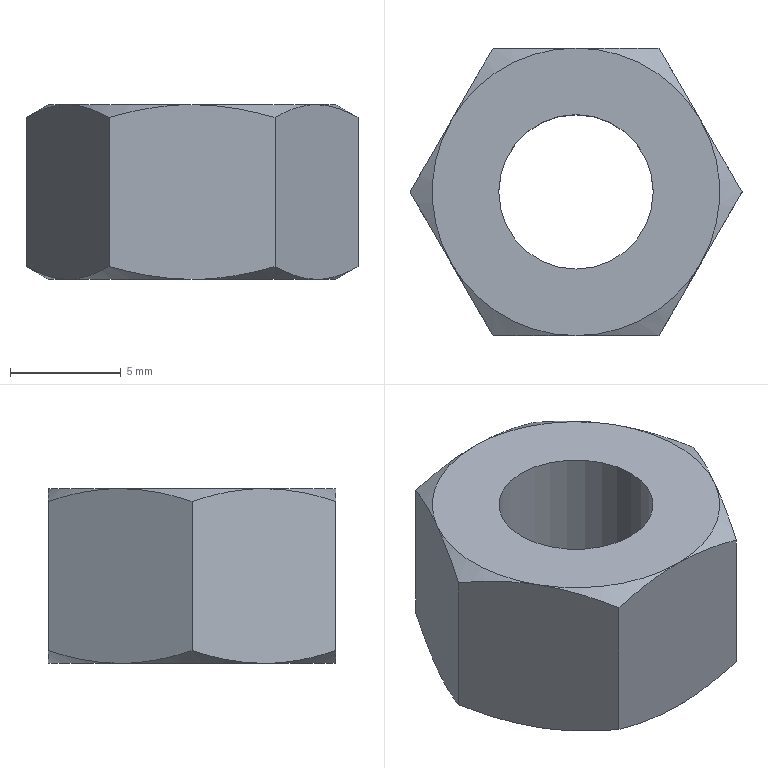Part | STEP file | 冲床-300配套压波_id202_x_t | 1 solid | 21 faces | box 15.011 x 13 x 7.9 mm | volume 848.643 mm3 | cone 12 | plane 8 | cylinder 1 | commonest cylinder face diameters 6.985 x1
STEP:
#1=CARTESIAN_POINT('',(1810.629,-81.75,123.));
#2=VERTEX_POINT('',#1);
#3=CARTESIAN_POINT('',(1805.,-78.5,123.));
#4=VERTEX_POINT('',#3);
#5=CARTESIAN_POINT('',(1805.,-85.,123.));
#6=DIRECTION('',(0.,0.,1.));
#7=DIRECTION('',(1.,0.,0.));
#8=AXIS2_PLACEMENT_3D('',#5,#6,#7);
#9=CIRCLE('',#8,6.5);
#10=EDGE_CURVE('',#2,#4,#9,.T.);
#11=ORIENTED_EDGE('',*,*,#10,.F.);
#12=CARTESIAN_POINT('',(1810.629,-88.25,123.));
#13=VERTEX_POINT('',#12);
#14=CARTESIAN_POINT('',(1805.,-85.,123.));
#15=DIRECTION('',(0.,0.,1.));
#16=DIRECTION('',(1.,0.,0.));
#17=AXIS2_PLACEMENT_3D('',#14,#15,#16);
#18=CIRCLE('',#17,6.5);
#19=EDGE_CURVE('',#13,#2,#18,.T.);
#20=ORIENTED_EDGE('',*,*,#19,.F.);
#21=CARTESIAN_POINT('',(1805.,-91.5,123.));
#22=VERTEX_POINT('',#21);
#23=CARTESIAN_POINT('',(1805.,-85.,123.));
#24=DIRECTION('',(0.,0.,1.));
#25=DIRECTION('',(1.,0.,0.));
#26=AXIS2_PLACEMENT_3D('',#23,#24,#25);
#27=CIRCLE('',#26,6.5);
#28=EDGE_CURVE('',#22,#13,#27,.T.);
#29=ORIENTED_EDGE('',*,*,#28,.F.);
#30=CARTESIAN_POINT('',(1799.371,-88.25,123.));
#31=VERTEX_POINT('',#30);
#32=CARTESIAN_POINT('',(1805.,-85.,123.));
#33=DIRECTION('',(0.,0.,1.));
#34=DIRECTION('',(1.,0.,0.));
#35=AXIS2_PLACEMENT_3D('',#32,#33,#34);
#36=CIRCLE('',#35,6.5);
#37=EDGE_CURVE('',#31,#22,#36,.T.);
#38=ORIENTED_EDGE('',*,*,#37,.F.);
#39=CARTESIAN_POINT('',(1799.371,-81.75,123.));
#40=VERTEX_POINT('',#39);
#41=CARTESIAN_POINT('',(1805.,-85.,123.));
#42=DIRECTION('',(0.,0.,1.));
#43=DIRECTION('',(1.,0.,0.));
#44=AXIS2_PLACEMENT_3D('',#41,#42,#43);
#45=CIRCLE('',#44,6.5);
#46=EDGE_CURVE('',#40,#31,#45,.T.);
#47=ORIENTED_EDGE('',*,*,#46,.F.);
#48=CARTESIAN_POINT('',(1805.,-85.,123.));
#49=DIRECTION('',(0.,0.,1.));
#50=DIRECTION('',(1.,0.,0.));
#51=AXIS2_PLACEMENT_3D('',#48,#49,#50);
#52=CIRCLE('',#51,6.5);
#53=EDGE_CURVE('',#4,#40,#52,.T.);
#54=ORIENTED_EDGE('',*,*,#53,.F.);
#55=EDGE_LOOP('',(#11,#20,#29,#38,#47,#54));
#56=FACE_BOUND('',#55,.T.);
#57=CARTESIAN_POINT('',(1801.507,-85.,123.));
#58=VERTEX_POINT('',#57);
#59=CARTESIAN_POINT('',(1805.,-85.,123.));
#60=DIRECTION('',(0.,0.,1.));
#61=DIRECTION('',(-1.,0.,0.));
#62=AXIS2_PLACEMENT_3D('',#59,#60,#61);
#63=CIRCLE('',#62,3.493);
#64=EDGE_CURVE('',#58,#58,#63,.T.);
#65=ORIENTED_EDGE('',*,*,#64,.T.);
#66=EDGE_LOOP('',(#65));
#67=FACE_BOUND('',#66,.T.);
#68=CARTESIAN_POINT('',(1805.,-72.,123.));
#69=DIRECTION('',(0.,0.,-1.));
#70=DIRECTION('',(-1.,0.,0.));
#71=AXIS2_PLACEMENT_3D('',#68,#69,#70);
#72=PLANE('',#71);
#73=ADVANCED_FACE('',(#56,#67),#72,.T.);
#74=CARTESIAN_POINT('',(1810.629,-88.25,130.9));
#75=VERTEX_POINT('',#74);
#76=CARTESIAN_POINT('',(1810.629,-81.75,130.9));
#77=VERTEX_POINT('',#76);
#78=CARTESIAN_POINT('',(1805.,-85.,130.9));
#79=DIRECTION('',(0.,0.,1.));
#80=DIRECTION('',(1.,0.,0.));
#81=AXIS2_PLACEMENT_3D('',#78,#79,#80);
#82=CIRCLE('',#81,6.5);
#83=EDGE_CURVE('',#75,#77,#82,.T.);
#84=ORIENTED_EDGE('',*,*,#83,.T.);
#85=CARTESIAN_POINT('',(1805.,-78.5,130.9));
#86=VERTEX_POINT('',#85);
#87=CARTESIAN_POINT('',(1805.,-85.,130.9));
#88=DIRECTION('',(0.,0.,1.));
#89=DIRECTION('',(1.,0.,0.));
#90=AXIS2_PLACEMENT_3D('',#87,#88,#89);
#91=CIRCLE('',#90,6.5);
#92=EDGE_CURVE('',#77,#86,#91,.T.);
#93=ORIENTED_EDGE('',*,*,#92,.T.);
#94=CARTESIAN_POINT('',(1799.371,-81.75,130.9));
#95=VERTEX_POINT('',#94);
#96=CARTESIAN_POINT('',(1805.,-85.,130.9));
#97=DIRECTION('',(0.,0.,1.));
#98=DIRECTION('',(1.,0.,0.));
#99=AXIS2_PLACEMENT_3D('',#96,#97,#98);
#100=CIRCLE('',#99,6.5);
#101=EDGE_CURVE('',#86,#95,#100,.T.);
#102=ORIENTED_EDGE('',*,*,#101,.T.);
#103=CARTESIAN_POINT('',(1799.371,-88.25,130.9));
#104=VERTEX_POINT('',#103);
#105=CARTESIAN_POINT('',(1805.,-85.,130.9));
#106=DIRECTION('',(0.,0.,1.));
#107=DIRECTION('',(1.,0.,0.));
#108=AXIS2_PLACEMENT_3D('',#105,#106,#107);
#109=CIRCLE('',#108,6.5);
#110=EDGE_CURVE('',#95,#104,#109,.T.);
#111=ORIENTED_EDGE('',*,*,#110,.T.);
#112=CARTESIAN_POINT('',(1805.,-91.5,130.9));
#113=VERTEX_POINT('',#112);
#114=CARTESIAN_POINT('',(1805.,-85.,130.9));
#115=DIRECTION('',(0.,0.,1.));
#116=DIRECTION('',(1.,0.,0.));
#117=AXIS2_PLACEMENT_3D('',#114,#115,#116);
#118=CIRCLE('',#117,6.5);
#119=EDGE_CURVE('',#104,#113,#118,.T.);
#120=ORIENTED_EDGE('',*,*,#119,.T.);
#121=CARTESIAN_POINT('',(1805.,-85.,130.9));
#122=DIRECTION('',(0.,0.,1.));
#123=DIRECTION('',(1.,0.,0.));
#124=AXIS2_PLACEMENT_3D('',#121,#122,#123);
#125=CIRCLE('',#124,6.5);
#126=EDGE_CURVE('',#113,#75,#125,.T.);
#127=ORIENTED_EDGE('',*,*,#126,.T.);
#128=EDGE_LOOP('',(#84,#93,#102,#111,#120,#127));
#129=FACE_BOUND('',#128,.T.);
#130=CARTESIAN_POINT('',(1801.507,-85.,130.9));
#131=VERTEX_POINT('',#130);
#132=CARTESIAN_POINT('',(1805.,-85.,130.9));
#133=DIRECTION('',(0.,0.,1.));
#134=DIRECTION('',(-1.,0.,0.));
#135=AXIS2_PLACEMENT_3D('',#132,#133,#134);
#136=CIRCLE('',#135,3.493);
#137=EDGE_CURVE('',#131,#131,#136,.T.);
#138=ORIENTED_EDGE('',*,*,#137,.F.);
#139=EDGE_LOOP('',(#138));
#140=FACE_BOUND('',#139,.T.);
#141=CARTESIAN_POINT('',(1805.,-72.,130.9));
#142=DIRECTION('',(0.,0.,-1.));
#143=DIRECTION('',(-1.,0.,0.));
#144=AXIS2_PLACEMENT_3D('',#141,#142,#143);
#145=PLANE('',#144);
#146=ADVANCED_FACE('',(#129,#140),#145,.F.);
#147=CARTESIAN_POINT('',(1797.494,-85.,123.581));
#148=VERTEX_POINT('',#147);
#149=CARTESIAN_POINT('',(1797.494,-85.,130.319));
#150=VERTEX_POINT('',#149);
#151=CARTESIAN_POINT('',(1797.494,-85.,123.));
#152=DIRECTION('',(0.,0.,1.));
#153=VECTOR('',#152,1.);
#154=LINE('',#151,#153);
#155=EDGE_CURVE('',#148,#150,#154,.T.);
#156=ORIENTED_EDGE('',*,*,#155,.T.);
#157=CARTESIAN_POINT('',(1797.494,-85.,130.319));
#158=CARTESIAN_POINT('',(1798.108,-83.937,130.674));
#159=CARTESIAN_POINT('',(1798.731,-82.857,130.9));
#160=CARTESIAN_POINT('',(1799.371,-81.75,130.9));
#161=B_SPLINE_CURVE_WITH_KNOTS('',3,(#157,#158,#159,#160),.UNSPECIFIED.,.F.,.F.,(4,4),(0.,1.),.UNSPECIFIED.);
#162=EDGE_CURVE('',#150,#95,#161,.T.);
#163=ORIENTED_EDGE('',*,*,#162,.T.);
#164=CARTESIAN_POINT('',(1801.247,-78.5,130.319));
#165=VERTEX_POINT('',#164);
#166=CARTESIAN_POINT('',(1799.371,-81.75,130.9));
#167=CARTESIAN_POINT('',(1800.008,-80.647,130.9));
#168=CARTESIAN_POINT('',(1800.635,-79.561,130.673));
#169=CARTESIAN_POINT('',(1801.247,-78.5,130.319));
#170=B_SPLINE_CURVE_WITH_KNOTS('',3,(#166,#167,#168,#169),.UNSPECIFIED.,.F.,.F.,(4,4),(0.,1.),.UNSPECIFIED.);
#171=EDGE_CURVE('',#95,#165,#170,.T.);
#172=ORIENTED_EDGE('',*,*,#171,.T.);
#173=CARTESIAN_POINT('',(1801.247,-78.5,123.581));
#174=VERTEX_POINT('',#173);
#175=CARTESIAN_POINT('',(1801.247,-78.5,123.));
#176=DIRECTION('',(0.,0.,1.));
#177=VECTOR('',#176,1.);
#178=LINE('',#175,#177);
#179=EDGE_CURVE('',#174,#165,#178,.T.);
#180=ORIENTED_EDGE('',*,*,#179,.F.);
#181=CARTESIAN_POINT('',(1801.247,-78.5,123.581));
#182=CARTESIAN_POINT('',(1800.633,-79.563,123.226));
#183=CARTESIAN_POINT('',(1800.01,-80.643,123.));
#184=CARTESIAN_POINT('',(1799.371,-81.75,123.));
#185=B_SPLINE_CURVE_WITH_KNOTS('',3,(#181,#182,#183,#184),.UNSPECIFIED.,.F.,.F.,(4,4),(0.,1.),.UNSPECIFIED.);
#186=EDGE_CURVE('',#174,#40,#185,.T.);
#187=ORIENTED_EDGE('',*,*,#186,.T.);
#188=CARTESIAN_POINT('',(1799.371,-81.75,123.));
#189=CARTESIAN_POINT('',(1798.734,-82.853,123.));
#190=CARTESIAN_POINT('',(1798.107,-83.939,123.227));
#191=CARTESIAN_POINT('',(1797.494,-85.,123.581));
#192=B_SPLINE_CURVE_WITH_KNOTS('',3,(#188,#189,#190,#191),.UNSPECIFIED.,.F.,.F.,(4,4),(0.,1.),.UNSPECIFIED.);
#193=EDGE_CURVE('',#40,#148,#192,.T.);
#194=ORIENTED_EDGE('',*,*,#193,.T.);
#195=EDGE_LOOP('',(#156,#163,#172,#180,#187,#194));
#196=FACE_OUTER_BOUND('',#195,.T.);
#197=CARTESIAN_POINT('',(1801.247,-78.5,123.));
#198=DIRECTION('',(-0.866,0.5,0.));
#199=DIRECTION('',(0.5,0.866,0.));
#200=AXIS2_PLACEMENT_3D('',#197,#198,#199);
#201=PLANE('',#200);
#202=ADVANCED_FACE('',(#196),#201,.T.);
#203=CARTESIAN_POINT('',(1801.247,-91.5,123.581));
#204=VERTEX_POINT('',#203);
#205=CARTESIAN_POINT('',(1801.247,-91.5,130.319));
#206=VERTEX_POINT('',#205);
#207=CARTESIAN_POINT('',(1801.247,-91.5,123.));
#208=DIRECTION('',(0.,0.,1.));
#209=VECTOR('',#208,1.);
#210=LINE('',#207,#209);
#211=EDGE_CURVE('',#204,#206,#210,.T.);
#212=ORIENTED_EDGE('',*,*,#211,.T.);
#213=CARTESIAN_POINT('',(1801.247,-91.5,130.319));
#214=CARTESIAN_POINT('',(1800.633,-90.437,130.674));
#215=CARTESIAN_POINT('',(1800.01,-89.357,130.9));
#216=CARTESIAN_POINT('',(1799.371,-88.25,130.9));
#217=B_SPLINE_CURVE_WITH_KNOTS('',3,(#213,#214,#215,#216),.UNSPECIFIED.,.F.,.F.,(4,4),(0.,1.),.UNSPECIFIED.);
#218=EDGE_CURVE('',#206,#104,#217,.T.);
#219=ORIENTED_EDGE('',*,*,#218,.T.);
#220=CARTESIAN_POINT('',(1799.371,-88.25,130.9));
#221=CARTESIAN_POINT('',(1798.734,-87.147,130.9));
#222=CARTESIAN_POINT('',(1798.107,-86.061,130.673));
#223=CARTESIAN_POINT('',(1797.494,-85.,130.319));
#224=B_SPLINE_CURVE_WITH_KNOTS('',3,(#220,#221,#222,#223),.UNSPECIFIED.,.F.,.F.,(4,4),(0.,1.),.UNSPECIFIED.);
#225=EDGE_CURVE('',#104,#150,#224,.T.);
#226=ORIENTED_EDGE('',*,*,#225,.T.);
#227=ORIENTED_EDGE('',*,*,#155,.F.);
#228=CARTESIAN_POINT('',(1797.494,-85.,123.581));
#229=CARTESIAN_POINT('',(1798.108,-86.063,123.226));
#230=CARTESIAN_POINT('',(1798.731,-87.143,123.));
#231=CARTESIAN_POINT('',(1799.371,-88.25,123.));
#232=B_SPLINE_CURVE_WITH_KNOTS('',3,(#228,#229,#230,#231),.UNSPECIFIED.,.F.,.F.,(4,4),(0.,1.),.UNSPECIFIED.);
#233=EDGE_CURVE('',#148,#31,#232,.T.);
#234=ORIENTED_EDGE('',*,*,#233,.T.);
#235=CARTESIAN_POINT('',(1799.371,-88.25,123.));
#236=CARTESIAN_POINT('',(1800.008,-89.353,123.));
#237=CARTESIAN_POINT('',(1800.635,-90.439,123.227));
#238=CARTESIAN_POINT('',(1801.247,-91.5,123.581));
#239=B_SPLINE_CURVE_WITH_KNOTS('',3,(#235,#236,#237,#238),.UNSPECIFIED.,.F.,.F.,(4,4),(0.,1.),.UNSPECIFIED.);
#240=EDGE_CURVE('',#31,#204,#239,.T.);
#241=ORIENTED_EDGE('',*,*,#240,.T.);
#242=EDGE_LOOP('',(#212,#219,#226,#227,#234,#241));
#243=FACE_OUTER_BOUND('',#242,.T.);
#244=CARTESIAN_POINT('',(1797.494,-85.,123.));
#245=DIRECTION('',(-0.866,-0.5,0.));
#246=DIRECTION('',(-0.5,0.866,0.));
#247=AXIS2_PLACEMENT_3D('',#244,#245,#246);
#248=PLANE('',#247);
#249=ADVANCED_FACE('',(#243),#248,.T.);
#250=CARTESIAN_POINT('',(1808.753,-91.5,123.581));
#251=VERTEX_POINT('',#250);
#252=CARTESIAN_POINT('',(1808.753,-91.5,130.319));
#253=VERTEX_POINT('',#252);
#254=CARTESIAN_POINT('',(1808.753,-91.5,123.));
#255=DIRECTION('',(0.,0.,1.));
#256=VECTOR('',#255,1.);
#257=LINE('',#254,#256);
#258=EDGE_CURVE('',#251,#253,#257,.T.);
#259=ORIENTED_EDGE('',*,*,#258,.T.);
#260=CARTESIAN_POINT('',(1808.753,-91.5,130.319));
#261=CARTESIAN_POINT('',(1807.532,-91.5,130.672));
#262=CARTESIAN_POINT('',(1806.268,-91.5,130.9));
#263=CARTESIAN_POINT('',(1805.,-91.5,130.9));
#264=B_SPLINE_CURVE_WITH_KNOTS('',3,(#260,#261,#262,#263),.UNSPECIFIED.,.F.,.F.,(4,4),(0.,1.),.UNSPECIFIED.);
#265=EDGE_CURVE('',#253,#113,#264,.T.);
#266=ORIENTED_EDGE('',*,*,#265,.T.);
#267=CARTESIAN_POINT('',(1805.,-91.5,130.9));
#268=CARTESIAN_POINT('',(1803.731,-91.5,130.9));
#269=CARTESIAN_POINT('',(1802.461,-91.5,130.67));
#270=CARTESIAN_POINT('',(1801.247,-91.5,130.319));
#271=B_SPLINE_CURVE_WITH_KNOTS('',3,(#267,#268,#269,#270),.UNSPECIFIED.,.F.,.F.,(4,4),(0.,1.),.UNSPECIFIED.);
#272=EDGE_CURVE('',#113,#206,#271,.T.);
#273=ORIENTED_EDGE('',*,*,#272,.T.);
#274=ORIENTED_EDGE('',*,*,#211,.F.);
#275=CARTESIAN_POINT('',(1801.247,-91.5,123.581));
#276=CARTESIAN_POINT('',(1802.461,-91.5,123.23));
#277=CARTESIAN_POINT('',(1803.731,-91.5,123.));
#278=CARTESIAN_POINT('',(1805.,-91.5,123.));
#279=B_SPLINE_CURVE_WITH_KNOTS('',3,(#275,#276,#277,#278),.UNSPECIFIED.,.F.,.F.,(4,4),(0.,1.),.UNSPECIFIED.);
#280=EDGE_CURVE('',#204,#22,#279,.T.);
#281=ORIENTED_EDGE('',*,*,#280,.T.);
#282=CARTESIAN_POINT('',(1805.,-91.5,123.));
#283=CARTESIAN_POINT('',(1806.268,-91.5,123.));
#284=CARTESIAN_POINT('',(1807.532,-91.5,123.228));
#285=CARTESIAN_POINT('',(1808.753,-91.5,123.581));
#286=B_SPLINE_CURVE_WITH_KNOTS('',3,(#282,#283,#284,#285),.UNSPECIFIED.,.F.,.F.,(4,4),(0.,1.),.UNSPECIFIED.);
#287=EDGE_CURVE('',#22,#251,#286,.T.);
#288=ORIENTED_EDGE('',*,*,#287,.T.);
#289=EDGE_LOOP('',(#259,#266,#273,#274,#281,#288));
#290=FACE_OUTER_BOUND('',#289,.T.);
#291=CARTESIAN_POINT('',(1801.247,-91.5,123.));
#292=DIRECTION('',(0.,-1.,0.));
#293=DIRECTION('',(0.,0.,1.));
#294=AXIS2_PLACEMENT_3D('',#291,#292,#293);
#295=PLANE('',#294);
#296=ADVANCED_FACE('',(#290),#295,.T.);
#297=CARTESIAN_POINT('',(1812.506,-85.,123.581));
#298=VERTEX_POINT('',#297);
#299=CARTESIAN_POINT('',(1812.506,-85.,130.319));
#300=VERTEX_POINT('',#299);
#301=CARTESIAN_POINT('',(1812.506,-85.,123.));
#302=DIRECTION('',(0.,0.,1.));
#303=VECTOR('',#302,1.);
#304=LINE('',#301,#303);
#305=EDGE_CURVE('',#298,#300,#304,.T.);
#306=ORIENTED_EDGE('',*,*,#305,.T.);
#307=CARTESIAN_POINT('',(1812.506,-85.,130.319));
#308=CARTESIAN_POINT('',(1811.892,-86.063,130.674));
#309=CARTESIAN_POINT('',(1811.269,-87.143,130.9));
#310=CARTESIAN_POINT('',(1810.629,-88.25,130.9));
#311=B_SPLINE_CURVE_WITH_KNOTS('',3,(#307,#308,#309,#310),.UNSPECIFIED.,.F.,.F.,(4,4),(0.,1.),.UNSPECIFIED.);
#312=EDGE_CURVE('',#300,#75,#311,.T.);
#313=ORIENTED_EDGE('',*,*,#312,.T.);
#314=CARTESIAN_POINT('',(1810.629,-88.25,130.9));
#315=CARTESIAN_POINT('',(1809.992,-89.353,130.9));
#316=CARTESIAN_POINT('',(1809.365,-90.439,130.673));
#317=CARTESIAN_POINT('',(1808.753,-91.5,130.319));
#318=B_SPLINE_CURVE_WITH_KNOTS('',3,(#314,#315,#316,#317),.UNSPECIFIED.,.F.,.F.,(4,4),(0.,1.),.UNSPECIFIED.);
#319=EDGE_CURVE('',#75,#253,#318,.T.);
#320=ORIENTED_EDGE('',*,*,#319,.T.);
#321=ORIENTED_EDGE('',*,*,#258,.F.);
#322=CARTESIAN_POINT('',(1808.753,-91.5,123.581));
#323=CARTESIAN_POINT('',(1809.367,-90.437,123.226));
#324=CARTESIAN_POINT('',(1809.99,-89.357,123.));
#325=CARTESIAN_POINT('',(1810.629,-88.25,123.));
#326=B_SPLINE_CURVE_WITH_KNOTS('',3,(#322,#323,#324,#325),.UNSPECIFIED.,.F.,.F.,(4,4),(0.,1.),.UNSPECIFIED.);
#327=EDGE_CURVE('',#251,#13,#326,.T.);
#328=ORIENTED_EDGE('',*,*,#327,.T.);
#329=CARTESIAN_POINT('',(1810.629,-88.25,123.));
#330=CARTESIAN_POINT('',(1811.266,-87.147,123.));
#331=CARTESIAN_POINT('',(1811.893,-86.061,123.227));
#332=CARTESIAN_POINT('',(1812.506,-85.,123.581));
#333=B_SPLINE_CURVE_WITH_KNOTS('',3,(#329,#330,#331,#332),.UNSPECIFIED.,.F.,.F.,(4,4),(0.,1.),.UNSPECIFIED.);
#334=EDGE_CURVE('',#13,#298,#333,.T.);
#335=ORIENTED_EDGE('',*,*,#334,.T.);
#336=EDGE_LOOP('',(#306,#313,#320,#321,#328,#335));
#337=FACE_OUTER_BOUND('',#336,.T.);
#338=CARTESIAN_POINT('',(1808.753,-91.5,123.));
#339=DIRECTION('',(0.866,-0.5,0.));
#340=DIRECTION('',(-0.5,-0.866,0.));
#341=AXIS2_PLACEMENT_3D('',#338,#339,#340);
#342=PLANE('',#341);
#343=ADVANCED_FACE('',(#337),#342,.T.);
#344=CARTESIAN_POINT('',(1808.753,-78.5,123.581));
#345=VERTEX_POINT('',#344);
#346=CARTESIAN_POINT('',(1808.753,-78.5,130.319));
#347=VERTEX_POINT('',#346);
#348=CARTESIAN_POINT('',(1808.753,-78.5,123.));
#349=DIRECTION('',(0.,0.,1.));
#350=VECTOR('',#349,1.);
#351=LINE('',#348,#350);
#352=EDGE_CURVE('',#345,#347,#351,.T.);
#353=ORIENTED_EDGE('',*,*,#352,.T.);
#354=CARTESIAN_POINT('',(1808.753,-78.5,130.319));
#355=CARTESIAN_POINT('',(1809.367,-79.563,130.674));
#356=CARTESIAN_POINT('',(1809.99,-80.643,130.9));
#357=CARTESIAN_POINT('',(1810.629,-81.75,130.9));
#358=B_SPLINE_CURVE_WITH_KNOTS('',3,(#354,#355,#356,#357),.UNSPECIFIED.,.F.,.F.,(4,4),(0.,1.),.UNSPECIFIED.);
#359=EDGE_CURVE('',#347,#77,#358,.T.);
#360=ORIENTED_EDGE('',*,*,#359,.T.);
#361=CARTESIAN_POINT('',(1810.629,-81.75,130.9));
#362=CARTESIAN_POINT('',(1811.266,-82.853,130.9));
#363=CARTESIAN_POINT('',(1811.893,-83.939,130.673));
#364=CARTESIAN_POINT('',(1812.506,-85.,130.319));
#365=B_SPLINE_CURVE_WITH_KNOTS('',3,(#361,#362,#363,#364),.UNSPECIFIED.,.F.,.F.,(4,4),(0.,1.),.UNSPECIFIED.);
#366=EDGE_CURVE('',#77,#300,#365,.T.);
#367=ORIENTED_EDGE('',*,*,#366,.T.);
#368=ORIENTED_EDGE('',*,*,#305,.F.);
#369=CARTESIAN_POINT('',(1812.506,-85.,123.581));
#370=CARTESIAN_POINT('',(1811.892,-83.937,123.226));
#371=CARTESIAN_POINT('',(1811.269,-82.857,123.));
#372=CARTESIAN_POINT('',(1810.629,-81.75,123.));
#373=B_SPLINE_CURVE_WITH_KNOTS('',3,(#369,#370,#371,#372),.UNSPECIFIED.,.F.,.F.,(4,4),(0.,1.),.UNSPECIFIED.);
#374=EDGE_CURVE('',#298,#2,#373,.T.);
#375=ORIENTED_EDGE('',*,*,#374,.T.);
#376=CARTESIAN_POINT('',(1810.629,-81.75,123.));
#377=CARTESIAN_POINT('',(1809.992,-80.647,123.));
#378=CARTESIAN_POINT('',(1809.365,-79.561,123.227));
#379=CARTESIAN_POINT('',(1808.753,-78.5,123.581));
#380=B_SPLINE_CURVE_WITH_KNOTS('',3,(#376,#377,#378,#379),.UNSPECIFIED.,.F.,.F.,(4,4),(0.,1.),.UNSPECIFIED.);
#381=EDGE_CURVE('',#2,#345,#380,.T.);
#382=ORIENTED_EDGE('',*,*,#381,.T.);
#383=EDGE_LOOP('',(#353,#360,#367,#368,#375,#382));
#384=FACE_OUTER_BOUND('',#383,.T.);
#385=CARTESIAN_POINT('',(1812.506,-85.,123.));
#386=DIRECTION('',(0.866,0.5,0.));
#387=DIRECTION('',(0.5,-0.866,0.));
#388=AXIS2_PLACEMENT_3D('',#385,#386,#387);
#389=PLANE('',#388);
#390=ADVANCED_FACE('',(#384),#389,.T.);
#391=ORIENTED_EDGE('',*,*,#179,.T.);
#392=CARTESIAN_POINT('',(1801.247,-78.5,130.319));
#393=CARTESIAN_POINT('',(1802.461,-78.5,130.67));
#394=CARTESIAN_POINT('',(1803.731,-78.5,130.9));
#395=CARTESIAN_POINT('',(1805.,-78.5,130.9));
#396=B_SPLINE_CURVE_WITH_KNOTS('',3,(#392,#393,#394,#395),.UNSPECIFIED.,.F.,.F.,(4,4),(0.,1.),.UNSPECIFIED.);
#397=EDGE_CURVE('',#165,#86,#396,.T.);
#398=ORIENTED_EDGE('',*,*,#397,.T.);
#399=CARTESIAN_POINT('',(1805.,-78.5,130.9));
#400=CARTESIAN_POINT('',(1806.268,-78.5,130.9));
#401=CARTESIAN_POINT('',(1807.532,-78.5,130.672));
#402=CARTESIAN_POINT('',(1808.753,-78.5,130.319));
#403=B_SPLINE_CURVE_WITH_KNOTS('',3,(#399,#400,#401,#402),.UNSPECIFIED.,.F.,.F.,(4,4),(0.,1.),.UNSPECIFIED.);
#404=EDGE_CURVE('',#86,#347,#403,.T.);
#405=ORIENTED_EDGE('',*,*,#404,.T.);
#406=ORIENTED_EDGE('',*,*,#352,.F.);
#407=CARTESIAN_POINT('',(1808.753,-78.5,123.581));
#408=CARTESIAN_POINT('',(1807.532,-78.5,123.228));
#409=CARTESIAN_POINT('',(1806.268,-78.5,123.));
#410=CARTESIAN_POINT('',(1805.,-78.5,123.));
#411=B_SPLINE_CURVE_WITH_KNOTS('',3,(#407,#408,#409,#410),.UNSPECIFIED.,.F.,.F.,(4,4),(0.,1.),.UNSPECIFIED.);
#412=EDGE_CURVE('',#345,#4,#411,.T.);
#413=ORIENTED_EDGE('',*,*,#412,.T.);
#414=CARTESIAN_POINT('',(1805.,-78.5,123.));
#415=CARTESIAN_POINT('',(1803.731,-78.5,123.));
#416=CARTESIAN_POINT('',(1802.461,-78.5,123.23));
#417=CARTESIAN_POINT('',(1801.247,-78.5,123.581));
#418=B_SPLINE_CURVE_WITH_KNOTS('',3,(#414,#415,#416,#417),.UNSPECIFIED.,.F.,.F.,(4,4),(0.,1.),.UNSPECIFIED.);
#419=EDGE_CURVE('',#4,#174,#418,.T.);
#420=ORIENTED_EDGE('',*,*,#419,.T.);
#421=EDGE_LOOP('',(#391,#398,#405,#406,#413,#420));
#422=FACE_OUTER_BOUND('',#421,.T.);
#423=CARTESIAN_POINT('',(1808.753,-78.5,123.));
#424=DIRECTION('',(0.,1.,0.));
#425=DIRECTION('',(0.,0.,-1.));
#426=AXIS2_PLACEMENT_3D('',#423,#424,#425);
#427=PLANE('',#426);
#428=ADVANCED_FACE('',(#422),#427,.T.);
#429=ORIENTED_EDGE('',*,*,#419,.F.);
#430=ORIENTED_EDGE('',*,*,#53,.T.);
#431=ORIENTED_EDGE('',*,*,#186,.F.);
#432=EDGE_LOOP('',(#429,#430,#431));
#433=FACE_OUTER_BOUND('',#432,.T.);
#434=CARTESIAN_POINT('',(1805.,-85.,123.581));
#435=DIRECTION('',(0.,0.,1.));
#436=DIRECTION('',(1.,0.,0.));
#437=AXIS2_PLACEMENT_3D('',#434,#435,#436);
#438=CONICAL_SURFACE('',#437,7.506,60.);
#439=ADVANCED_FACE('',(#433),#438,.T.);
#440=ORIENTED_EDGE('',*,*,#10,.T.);
#441=ORIENTED_EDGE('',*,*,#412,.F.);
#442=ORIENTED_EDGE('',*,*,#381,.F.);
#443=EDGE_LOOP('',(#440,#441,#442));
#444=FACE_OUTER_BOUND('',#443,.T.);
#445=CARTESIAN_POINT('',(1805.,-85.,123.581));
#446=DIRECTION('',(0.,0.,1.));
#447=DIRECTION('',(1.,0.,0.));
#448=AXIS2_PLACEMENT_3D('',#445,#446,#447);
#449=CONICAL_SURFACE('',#448,7.506,60.);
#450=ADVANCED_FACE('',(#444),#449,.T.);
#451=ORIENTED_EDGE('',*,*,#19,.T.);
#452=ORIENTED_EDGE('',*,*,#374,.F.);
#453=ORIENTED_EDGE('',*,*,#334,.F.);
#454=EDGE_LOOP('',(#451,#452,#453));
#455=FACE_OUTER_BOUND('',#454,.T.);
#456=CARTESIAN_POINT('',(1805.,-85.,123.581));
#457=DIRECTION('',(0.,0.,1.));
#458=DIRECTION('',(1.,0.,0.));
#459=AXIS2_PLACEMENT_3D('',#456,#457,#458);
#460=CONICAL_SURFACE('',#459,7.506,60.);
#461=ADVANCED_FACE('',(#455),#460,.T.);
#462=ORIENTED_EDGE('',*,*,#28,.T.);
#463=ORIENTED_EDGE('',*,*,#327,.F.);
#464=ORIENTED_EDGE('',*,*,#287,.F.);
#465=EDGE_LOOP('',(#462,#463,#464));
#466=FACE_OUTER_BOUND('',#465,.T.);
#467=CARTESIAN_POINT('',(1805.,-85.,123.581));
#468=DIRECTION('',(0.,0.,1.));
#469=DIRECTION('',(1.,0.,0.));
#470=AXIS2_PLACEMENT_3D('',#467,#468,#469);
#471=CONICAL_SURFACE('',#470,7.506,60.);
#472=ADVANCED_FACE('',(#466),#471,.T.);
#473=ORIENTED_EDGE('',*,*,#37,.T.);
#474=ORIENTED_EDGE('',*,*,#280,.F.);
#475=ORIENTED_EDGE('',*,*,#240,.F.);
#476=EDGE_LOOP('',(#473,#474,#475));
#477=FACE_OUTER_BOUND('',#476,.T.);
#478=CARTESIAN_POINT('',(1805.,-85.,123.581));
#479=DIRECTION('',(0.,0.,1.));
#480=DIRECTION('',(1.,0.,0.));
#481=AXIS2_PLACEMENT_3D('',#478,#479,#480);
#482=CONICAL_SURFACE('',#481,7.506,60.);
#483=ADVANCED_FACE('',(#477),#482,.T.);
#484=ORIENTED_EDGE('',*,*,#46,.T.);
#485=ORIENTED_EDGE('',*,*,#233,.F.);
#486=ORIENTED_EDGE('',*,*,#193,.F.);
#487=EDGE_LOOP('',(#484,#485,#486));
#488=FACE_OUTER_BOUND('',#487,.T.);
#489=CARTESIAN_POINT('',(1805.,-85.,123.581));
#490=DIRECTION('',(0.,0.,1.));
#491=DIRECTION('',(1.,0.,0.));
#492=AXIS2_PLACEMENT_3D('',#489,#490,#491);
#493=CONICAL_SURFACE('',#492,7.506,60.);
#494=ADVANCED_FACE('',(#488),#493,.T.);
#495=ORIENTED_EDGE('',*,*,#404,.F.);
#496=ORIENTED_EDGE('',*,*,#92,.F.);
#497=ORIENTED_EDGE('',*,*,#359,.F.);
#498=EDGE_LOOP('',(#495,#496,#497));
#499=FACE_OUTER_BOUND('',#498,.T.);
#500=CARTESIAN_POINT('',(1805.,-85.,130.9));
#501=DIRECTION('',(0.,0.,-1.));
#502=DIRECTION('',(-1.,0.,0.));
#503=AXIS2_PLACEMENT_3D('',#500,#501,#502);
#504=CONICAL_SURFACE('',#503,6.5,60.);
#505=ADVANCED_FACE('',(#499),#504,.T.);
#506=ORIENTED_EDGE('',*,*,#101,.F.);
#507=ORIENTED_EDGE('',*,*,#397,.F.);
#508=ORIENTED_EDGE('',*,*,#171,.F.);
#509=EDGE_LOOP('',(#506,#507,#508));
#510=FACE_OUTER_BOUND('',#509,.T.);
#511=CARTESIAN_POINT('',(1805.,-85.,130.9));
#512=DIRECTION('',(0.,0.,-1.));
#513=DIRECTION('',(-1.,0.,0.));
#514=AXIS2_PLACEMENT_3D('',#511,#512,#513);
#515=CONICAL_SURFACE('',#514,6.5,60.);
#516=ADVANCED_FACE('',(#510),#515,.T.);
#517=ORIENTED_EDGE('',*,*,#366,.F.);
#518=ORIENTED_EDGE('',*,*,#83,.F.);
#519=ORIENTED_EDGE('',*,*,#312,.F.);
#520=EDGE_LOOP('',(#517,#518,#519));
#521=FACE_OUTER_BOUND('',#520,.T.);
#522=CARTESIAN_POINT('',(1805.,-85.,130.9));
#523=DIRECTION('',(0.,0.,-1.));
#524=DIRECTION('',(-1.,0.,0.));
#525=AXIS2_PLACEMENT_3D('',#522,#523,#524);
#526=CONICAL_SURFACE('',#525,6.5,60.);
#527=ADVANCED_FACE('',(#521),#526,.T.);
#528=ORIENTED_EDGE('',*,*,#319,.F.);
#529=ORIENTED_EDGE('',*,*,#126,.F.);
#530=ORIENTED_EDGE('',*,*,#265,.F.);
#531=EDGE_LOOP('',(#528,#529,#530));
#532=FACE_OUTER_BOUND('',#531,.T.);
#533=CARTESIAN_POINT('',(1805.,-85.,130.9));
#534=DIRECTION('',(0.,0.,-1.));
#535=DIRECTION('',(-1.,0.,0.));
#536=AXIS2_PLACEMENT_3D('',#533,#534,#535);
#537=CONICAL_SURFACE('',#536,6.5,60.);
#538=ADVANCED_FACE('',(#532),#537,.T.);
#539=ORIENTED_EDGE('',*,*,#119,.F.);
#540=ORIENTED_EDGE('',*,*,#218,.F.);
#541=ORIENTED_EDGE('',*,*,#272,.F.);
#542=EDGE_LOOP('',(#539,#540,#541));
#543=FACE_OUTER_BOUND('',#542,.T.);
#544=CARTESIAN_POINT('',(1805.,-85.,130.9));
#545=DIRECTION('',(0.,0.,-1.));
#546=DIRECTION('',(-1.,0.,0.));
#547=AXIS2_PLACEMENT_3D('',#544,#545,#546);
#548=CONICAL_SURFACE('',#547,6.5,60.);
#549=ADVANCED_FACE('',(#543),#548,.T.);
#550=ORIENTED_EDGE('',*,*,#110,.F.);
#551=ORIENTED_EDGE('',*,*,#162,.F.);
#552=ORIENTED_EDGE('',*,*,#225,.F.);
#553=EDGE_LOOP('',(#550,#551,#552));
#554=FACE_OUTER_BOUND('',#553,.T.);
#555=CARTESIAN_POINT('',(1805.,-85.,130.9));
#556=DIRECTION('',(0.,0.,-1.));
#557=DIRECTION('',(-1.,0.,0.));
#558=AXIS2_PLACEMENT_3D('',#555,#556,#557);
#559=CONICAL_SURFACE('',#558,6.5,60.);
#560=ADVANCED_FACE('',(#554),#559,.T.);
#561=ORIENTED_EDGE('',*,*,#64,.F.);
#562=EDGE_LOOP('',(#561));
#563=FACE_BOUND('',#562,.T.);
#564=ORIENTED_EDGE('',*,*,#137,.T.);
#565=EDGE_LOOP('',(#564));
#566=FACE_BOUND('',#565,.T.);
#567=CARTESIAN_POINT('',(1805.,-85.,123.));
#568=DIRECTION('',(0.,0.,1.));
#569=DIRECTION('',(1.,0.,0.));
#570=AXIS2_PLACEMENT_3D('',#567,#568,#569);
#571=CYLINDRICAL_SURFACE('',#570,3.493);
#572=ADVANCED_FACE('',(#563,#566),#571,.F.);
#573=CLOSED_SHELL('',(#73,#146,#202,#249,#296,#343,#390,#428,#439,#450,#461,#472,#483,#494,#505,#516,#527,#538,#549,#560,#572));
#574=MANIFOLD_SOLID_BREP('',#573);
#575=(LENGTH_UNIT()NAMED_UNIT(*)SI_UNIT(.MILLI.,.METRE.));
#576=UNCERTAINTY_MEASURE_WITH_UNIT(LENGTH_MEASURE(0.0508),#575,'','');
#577=(NAMED_UNIT(*)PLANE_ANGLE_UNIT()SI_UNIT($,.RADIAN.));
#578=PLANE_ANGLE_MEASURE_WITH_UNIT(PLANE_ANGLE_MEASURE(0.01745),#577);
#579=DIMENSIONAL_EXPONENTS(0.,0.,0.,0.,0.,0.,0.);
#580=(CONVERSION_BASED_UNIT('DEGREE',#578)NAMED_UNIT(#579)PLANE_ANGLE_UNIT());
#581=(NAMED_UNIT(*)SI_UNIT($,.STERADIAN.)SOLID_ANGLE_UNIT());
#582=(GEOMETRIC_REPRESENTATION_CONTEXT(3)GLOBAL_UNCERTAINTY_ASSIGNED_CONTEXT((#576))GLOBAL_UNIT_ASSIGNED_CONTEXT((#575,#580,#581))REPRESENTATION_CONTEXT('',''));
#583=ADVANCED_BREP_SHAPE_REPRESENTATION('',(#574),#582);